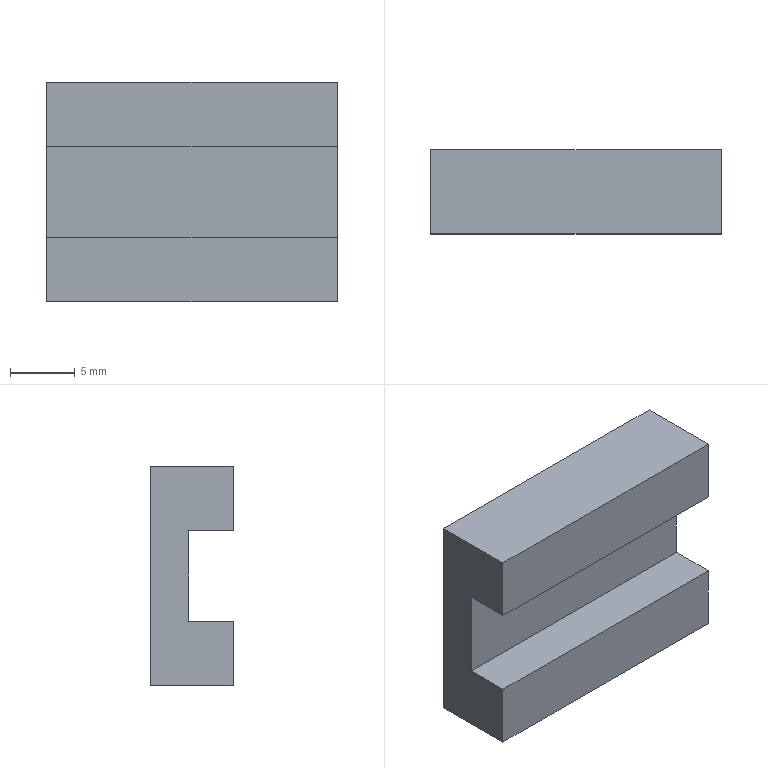Part | SolidWorks | features Extrusion 1, ICE 1 | 1 solid | 22 faces | box 22.5 x 6.5 x 17 mm | volume 1885 mm3 | plane 14 | cylinder 8 | commonest cylinder face diameters 2.635 x4 2.977 x4
STEP:
#1=CARTESIAN_POINT('',(-4.,3.047,4.441));
#2=VERTEX_POINT('',#1);
#3=CARTESIAN_POINT('',(-4.,3.047,7.076));
#4=VERTEX_POINT('',#3);
#5=CARTESIAN_POINT('',(-4.,3.047,5.759));
#6=DIRECTION('',(0.,1.,0.));
#7=DIRECTION('',(0.,0.,-1.));
#8=AXIS2_PLACEMENT_3D('',#5,#6,#7);
#9=CIRCLE('',#8,1.317);
#10=EDGE_CURVE('',#2,#4,#9,.T.);
#11=ORIENTED_EDGE('',*,*,#10,.F.);
#12=CARTESIAN_POINT('',(-4.,5.047,4.441));
#13=VERTEX_POINT('',#12);
#14=CARTESIAN_POINT('',(-4.,3.047,4.441));
#15=DIRECTION('',(0.,1.,0.));
#16=VECTOR('',#15,1000.);
#17=LINE('',#14,#16);
#18=EDGE_CURVE('',#2,#13,#17,.T.);
#19=ORIENTED_EDGE('',*,*,#18,.T.);
#20=CARTESIAN_POINT('',(-4.,5.047,7.076));
#21=VERTEX_POINT('',#20);
#22=CARTESIAN_POINT('',(-4.,5.047,5.759));
#23=DIRECTION('',(0.,1.,0.));
#24=DIRECTION('',(0.,0.,-1.));
#25=AXIS2_PLACEMENT_3D('',#22,#23,#24);
#26=CIRCLE('',#25,1.317);
#27=EDGE_CURVE('',#13,#21,#26,.T.);
#28=ORIENTED_EDGE('',*,*,#27,.T.);
#29=CARTESIAN_POINT('',(-4.,3.047,7.076));
#30=DIRECTION('',(0.,1.,0.));
#31=VECTOR('',#30,1000.);
#32=LINE('',#29,#31);
#33=EDGE_CURVE('',#4,#21,#32,.T.);
#34=ORIENTED_EDGE('',*,*,#33,.F.);
#35=EDGE_LOOP('',(#11,#19,#28,#34));
#36=FACE_OUTER_BOUND('',#35,.T.);
#37=CARTESIAN_POINT('',(-4.,3.047,5.759));
#38=DIRECTION('',(0.,1.,0.));
#39=DIRECTION('',(0.,0.,1.));
#40=AXIS2_PLACEMENT_3D('',#37,#38,#39);
#41=CYLINDRICAL_SURFACE('',#40,1.317);
#42=ADVANCED_FACE('',(#36),#41,.F.);
#43=CARTESIAN_POINT('',(4.,3.047,-7.73));
#44=VERTEX_POINT('',#43);
#45=CARTESIAN_POINT('',(4.,3.047,-4.753));
#46=VERTEX_POINT('',#45);
#47=CARTESIAN_POINT('',(4.,3.047,-6.241));
#48=DIRECTION('',(0.,1.,0.));
#49=DIRECTION('',(0.,0.,-1.));
#50=AXIS2_PLACEMENT_3D('',#47,#48,#49);
#51=CIRCLE('',#50,1.488);
#52=EDGE_CURVE('',#44,#46,#51,.T.);
#53=ORIENTED_EDGE('',*,*,#52,.F.);
#54=CARTESIAN_POINT('',(4.,5.047,-7.73));
#55=VERTEX_POINT('',#54);
#56=CARTESIAN_POINT('',(4.,3.047,-7.73));
#57=DIRECTION('',(0.,1.,0.));
#58=VECTOR('',#57,1000.);
#59=LINE('',#56,#58);
#60=EDGE_CURVE('',#44,#55,#59,.T.);
#61=ORIENTED_EDGE('',*,*,#60,.T.);
#62=CARTESIAN_POINT('',(4.,5.047,-4.753));
#63=VERTEX_POINT('',#62);
#64=CARTESIAN_POINT('',(4.,5.047,-6.241));
#65=DIRECTION('',(0.,1.,0.));
#66=DIRECTION('',(0.,0.,-1.));
#67=AXIS2_PLACEMENT_3D('',#64,#65,#66);
#68=CIRCLE('',#67,1.488);
#69=EDGE_CURVE('',#55,#63,#68,.T.);
#70=ORIENTED_EDGE('',*,*,#69,.T.);
#71=CARTESIAN_POINT('',(4.,3.047,-4.753));
#72=DIRECTION('',(0.,1.,0.));
#73=VECTOR('',#72,1000.);
#74=LINE('',#71,#73);
#75=EDGE_CURVE('',#46,#63,#74,.T.);
#76=ORIENTED_EDGE('',*,*,#75,.F.);
#77=EDGE_LOOP('',(#53,#61,#70,#76));
#78=FACE_OUTER_BOUND('',#77,.T.);
#79=CARTESIAN_POINT('',(4.,3.047,-6.241));
#80=DIRECTION('',(0.,1.,0.));
#81=DIRECTION('',(0.,0.,1.));
#82=AXIS2_PLACEMENT_3D('',#79,#80,#81);
#83=CYLINDRICAL_SURFACE('',#82,1.488);
#84=ADVANCED_FACE('',(#78),#83,.F.);
#85=CARTESIAN_POINT('',(-4.,3.047,-7.73));
#86=VERTEX_POINT('',#85);
#87=CARTESIAN_POINT('',(-4.,3.047,-4.753));
#88=VERTEX_POINT('',#87);
#89=CARTESIAN_POINT('',(-4.,3.047,-6.241));
#90=DIRECTION('',(0.,1.,0.));
#91=DIRECTION('',(0.,0.,1.));
#92=AXIS2_PLACEMENT_3D('',#89,#90,#91);
#93=CIRCLE('',#92,1.488);
#94=EDGE_CURVE('',#86,#88,#93,.T.);
#95=ORIENTED_EDGE('',*,*,#94,.F.);
#96=CARTESIAN_POINT('',(-4.,5.047,-7.73));
#97=VERTEX_POINT('',#96);
#98=CARTESIAN_POINT('',(-4.,3.047,-7.73));
#99=DIRECTION('',(0.,1.,0.));
#100=VECTOR('',#99,1000.);
#101=LINE('',#98,#100);
#102=EDGE_CURVE('',#86,#97,#101,.T.);
#103=ORIENTED_EDGE('',*,*,#102,.T.);
#104=CARTESIAN_POINT('',(-4.,5.047,-4.753));
#105=VERTEX_POINT('',#104);
#106=CARTESIAN_POINT('',(-4.,5.047,-6.241));
#107=DIRECTION('',(0.,1.,0.));
#108=DIRECTION('',(0.,0.,1.));
#109=AXIS2_PLACEMENT_3D('',#106,#107,#108);
#110=CIRCLE('',#109,1.488);
#111=EDGE_CURVE('',#97,#105,#110,.T.);
#112=ORIENTED_EDGE('',*,*,#111,.T.);
#113=CARTESIAN_POINT('',(-4.,3.047,-4.753));
#114=DIRECTION('',(0.,1.,0.));
#115=VECTOR('',#114,1000.);
#116=LINE('',#113,#115);
#117=EDGE_CURVE('',#88,#105,#116,.T.);
#118=ORIENTED_EDGE('',*,*,#117,.F.);
#119=EDGE_LOOP('',(#95,#103,#112,#118));
#120=FACE_OUTER_BOUND('',#119,.T.);
#121=CARTESIAN_POINT('',(-4.,3.047,-6.241));
#122=DIRECTION('',(0.,1.,0.));
#123=DIRECTION('',(0.,0.,1.));
#124=AXIS2_PLACEMENT_3D('',#121,#122,#123);
#125=CYLINDRICAL_SURFACE('',#124,1.488);
#126=ADVANCED_FACE('',(#120),#125,.F.);
#127=CARTESIAN_POINT('',(4.,3.047,4.441));
#128=VERTEX_POINT('',#127);
#129=CARTESIAN_POINT('',(4.,3.047,7.076));
#130=VERTEX_POINT('',#129);
#131=CARTESIAN_POINT('',(4.,3.047,5.759));
#132=DIRECTION('',(0.,1.,0.));
#133=DIRECTION('',(0.,0.,1.));
#134=AXIS2_PLACEMENT_3D('',#131,#132,#133);
#135=CIRCLE('',#134,1.317);
#136=EDGE_CURVE('',#128,#130,#135,.T.);
#137=ORIENTED_EDGE('',*,*,#136,.F.);
#138=CARTESIAN_POINT('',(4.,5.047,4.441));
#139=VERTEX_POINT('',#138);
#140=CARTESIAN_POINT('',(4.,3.047,4.441));
#141=DIRECTION('',(0.,1.,0.));
#142=VECTOR('',#141,1000.);
#143=LINE('',#140,#142);
#144=EDGE_CURVE('',#128,#139,#143,.T.);
#145=ORIENTED_EDGE('',*,*,#144,.T.);
#146=CARTESIAN_POINT('',(4.,5.047,7.076));
#147=VERTEX_POINT('',#146);
#148=CARTESIAN_POINT('',(4.,5.047,5.759));
#149=DIRECTION('',(0.,1.,0.));
#150=DIRECTION('',(0.,0.,1.));
#151=AXIS2_PLACEMENT_3D('',#148,#149,#150);
#152=CIRCLE('',#151,1.317);
#153=EDGE_CURVE('',#139,#147,#152,.T.);
#154=ORIENTED_EDGE('',*,*,#153,.T.);
#155=CARTESIAN_POINT('',(4.,3.047,7.076));
#156=DIRECTION('',(0.,1.,0.));
#157=VECTOR('',#156,1000.);
#158=LINE('',#155,#157);
#159=EDGE_CURVE('',#130,#147,#158,.T.);
#160=ORIENTED_EDGE('',*,*,#159,.F.);
#161=EDGE_LOOP('',(#137,#145,#154,#160));
#162=FACE_OUTER_BOUND('',#161,.T.);
#163=CARTESIAN_POINT('',(4.,3.047,5.759));
#164=DIRECTION('',(0.,1.,0.));
#165=DIRECTION('',(0.,0.,1.));
#166=AXIS2_PLACEMENT_3D('',#163,#164,#165);
#167=CYLINDRICAL_SURFACE('',#166,1.317);
#168=ADVANCED_FACE('',(#162),#167,.F.);
#169=CARTESIAN_POINT('',(-11.25,5.047,8.259));
#170=VERTEX_POINT('',#169);
#171=CARTESIAN_POINT('',(-11.25,-1.453,8.259));
#172=VERTEX_POINT('',#171);
#173=CARTESIAN_POINT('',(-11.25,5.047,8.259));
#174=DIRECTION('',(0.,-1.,0.));
#175=VECTOR('',#174,1000.);
#176=LINE('',#173,#175);
#177=EDGE_CURVE('',#170,#172,#176,.T.);
#178=ORIENTED_EDGE('',*,*,#177,.T.);
#179=CARTESIAN_POINT('',(11.25,-1.453,8.259));
#180=VERTEX_POINT('',#179);
#181=CARTESIAN_POINT('',(11.25,-1.453,8.259));
#182=DIRECTION('',(-1.,0.,0.));
#183=VECTOR('',#182,1000.);
#184=LINE('',#181,#183);
#185=EDGE_CURVE('',#180,#172,#184,.T.);
#186=ORIENTED_EDGE('',*,*,#185,.F.);
#187=CARTESIAN_POINT('',(11.25,5.047,8.259));
#188=VERTEX_POINT('',#187);
#189=CARTESIAN_POINT('',(11.25,5.047,8.259));
#190=DIRECTION('',(0.,-1.,0.));
#191=VECTOR('',#190,1000.);
#192=LINE('',#189,#191);
#193=EDGE_CURVE('',#188,#180,#192,.T.);
#194=ORIENTED_EDGE('',*,*,#193,.F.);
#195=CARTESIAN_POINT('',(11.25,5.047,8.259));
#196=DIRECTION('',(-1.,0.,0.));
#197=VECTOR('',#196,1000.);
#198=LINE('',#195,#197);
#199=EDGE_CURVE('',#188,#170,#198,.T.);
#200=ORIENTED_EDGE('',*,*,#199,.T.);
#201=EDGE_LOOP('',(#178,#186,#194,#200));
#202=FACE_OUTER_BOUND('',#201,.T.);
#203=CARTESIAN_POINT('',(11.25,5.047,8.259));
#204=DIRECTION('',(0.,0.,-1.));
#205=DIRECTION('',(0.,1.,0.));
#206=AXIS2_PLACEMENT_3D('',#203,#204,#205);
#207=PLANE('',#206);
#208=ADVANCED_FACE('',(#202),#207,.F.);
#209=CARTESIAN_POINT('',(-11.25,-1.453,3.259));
#210=VERTEX_POINT('',#209);
#211=CARTESIAN_POINT('',(-11.25,-1.453,8.259));
#212=DIRECTION('',(0.,0.,-1.));
#213=VECTOR('',#212,1000.);
#214=LINE('',#211,#213);
#215=EDGE_CURVE('',#172,#210,#214,.T.);
#216=ORIENTED_EDGE('',*,*,#215,.T.);
#217=CARTESIAN_POINT('',(11.25,-1.453,3.259));
#218=VERTEX_POINT('',#217);
#219=CARTESIAN_POINT('',(11.25,-1.453,3.259));
#220=DIRECTION('',(-1.,0.,0.));
#221=VECTOR('',#220,1000.);
#222=LINE('',#219,#221);
#223=EDGE_CURVE('',#218,#210,#222,.T.);
#224=ORIENTED_EDGE('',*,*,#223,.F.);
#225=CARTESIAN_POINT('',(11.25,-1.453,8.259));
#226=DIRECTION('',(0.,0.,-1.));
#227=VECTOR('',#226,1000.);
#228=LINE('',#225,#227);
#229=EDGE_CURVE('',#180,#218,#228,.T.);
#230=ORIENTED_EDGE('',*,*,#229,.F.);
#231=ORIENTED_EDGE('',*,*,#185,.T.);
#232=EDGE_LOOP('',(#216,#224,#230,#231));
#233=FACE_OUTER_BOUND('',#232,.T.);
#234=CARTESIAN_POINT('',(11.25,-1.453,8.259));
#235=DIRECTION('',(0.,1.,0.));
#236=DIRECTION('',(0.,0.,1.));
#237=AXIS2_PLACEMENT_3D('',#234,#235,#236);
#238=PLANE('',#237);
#239=ADVANCED_FACE('',(#233),#238,.F.);
#240=CARTESIAN_POINT('',(-11.25,2.047,3.259));
#241=VERTEX_POINT('',#240);
#242=CARTESIAN_POINT('',(-11.25,-1.453,3.259));
#243=DIRECTION('',(0.,1.,0.));
#244=VECTOR('',#243,1000.);
#245=LINE('',#242,#244);
#246=EDGE_CURVE('',#210,#241,#245,.T.);
#247=ORIENTED_EDGE('',*,*,#246,.T.);
#248=CARTESIAN_POINT('',(11.25,2.047,3.259));
#249=VERTEX_POINT('',#248);
#250=CARTESIAN_POINT('',(11.25,2.047,3.259));
#251=DIRECTION('',(-1.,0.,0.));
#252=VECTOR('',#251,1000.);
#253=LINE('',#250,#252);
#254=EDGE_CURVE('',#249,#241,#253,.T.);
#255=ORIENTED_EDGE('',*,*,#254,.F.);
#256=CARTESIAN_POINT('',(11.25,-1.453,3.259));
#257=DIRECTION('',(0.,1.,0.));
#258=VECTOR('',#257,1000.);
#259=LINE('',#256,#258);
#260=EDGE_CURVE('',#218,#249,#259,.T.);
#261=ORIENTED_EDGE('',*,*,#260,.F.);
#262=ORIENTED_EDGE('',*,*,#223,.T.);
#263=EDGE_LOOP('',(#247,#255,#261,#262));
#264=FACE_OUTER_BOUND('',#263,.T.);
#265=CARTESIAN_POINT('',(11.25,-1.453,3.259));
#266=DIRECTION('',(0.,0.,1.));
#267=DIRECTION('',(1.,0.,0.));
#268=AXIS2_PLACEMENT_3D('',#265,#266,#267);
#269=PLANE('',#268);
#270=ADVANCED_FACE('',(#264),#269,.F.);
#271=CARTESIAN_POINT('',(-11.25,2.047,-3.741));
#272=VERTEX_POINT('',#271);
#273=CARTESIAN_POINT('',(-11.25,2.047,3.259));
#274=DIRECTION('',(0.,0.,-1.));
#275=VECTOR('',#274,1000.);
#276=LINE('',#273,#275);
#277=EDGE_CURVE('',#241,#272,#276,.T.);
#278=ORIENTED_EDGE('',*,*,#277,.T.);
#279=CARTESIAN_POINT('',(11.25,2.047,-3.741));
#280=VERTEX_POINT('',#279);
#281=CARTESIAN_POINT('',(11.25,2.047,-3.741));
#282=DIRECTION('',(-1.,0.,0.));
#283=VECTOR('',#282,1000.);
#284=LINE('',#281,#283);
#285=EDGE_CURVE('',#280,#272,#284,.T.);
#286=ORIENTED_EDGE('',*,*,#285,.F.);
#287=CARTESIAN_POINT('',(11.25,2.047,3.259));
#288=DIRECTION('',(0.,0.,-1.));
#289=VECTOR('',#288,1000.);
#290=LINE('',#287,#289);
#291=EDGE_CURVE('',#249,#280,#290,.T.);
#292=ORIENTED_EDGE('',*,*,#291,.F.);
#293=ORIENTED_EDGE('',*,*,#254,.T.);
#294=EDGE_LOOP('',(#278,#286,#292,#293));
#295=FACE_OUTER_BOUND('',#294,.T.);
#296=CARTESIAN_POINT('',(11.25,2.047,3.259));
#297=DIRECTION('',(0.,1.,0.));
#298=DIRECTION('',(0.,0.,1.));
#299=AXIS2_PLACEMENT_3D('',#296,#297,#298);
#300=PLANE('',#299);
#301=ADVANCED_FACE('',(#295),#300,.F.);
#302=CARTESIAN_POINT('',(-11.25,-1.453,-3.741));
#303=VERTEX_POINT('',#302);
#304=CARTESIAN_POINT('',(-11.25,2.047,-3.741));
#305=DIRECTION('',(0.,-1.,0.));
#306=VECTOR('',#305,1000.);
#307=LINE('',#304,#306);
#308=EDGE_CURVE('',#272,#303,#307,.T.);
#309=ORIENTED_EDGE('',*,*,#308,.T.);
#310=CARTESIAN_POINT('',(11.25,-1.453,-3.741));
#311=VERTEX_POINT('',#310);
#312=CARTESIAN_POINT('',(11.25,-1.453,-3.741));
#313=DIRECTION('',(-1.,0.,0.));
#314=VECTOR('',#313,1000.);
#315=LINE('',#312,#314);
#316=EDGE_CURVE('',#311,#303,#315,.T.);
#317=ORIENTED_EDGE('',*,*,#316,.F.);
#318=CARTESIAN_POINT('',(11.25,2.047,-3.741));
#319=DIRECTION('',(0.,-1.,0.));
#320=VECTOR('',#319,1000.);
#321=LINE('',#318,#320);
#322=EDGE_CURVE('',#280,#311,#321,.T.);
#323=ORIENTED_EDGE('',*,*,#322,.F.);
#324=ORIENTED_EDGE('',*,*,#285,.T.);
#325=EDGE_LOOP('',(#309,#317,#323,#324));
#326=FACE_OUTER_BOUND('',#325,.T.);
#327=CARTESIAN_POINT('',(11.25,2.047,-3.741));
#328=DIRECTION('',(0.,0.,-1.));
#329=DIRECTION('',(0.,1.,0.));
#330=AXIS2_PLACEMENT_3D('',#327,#328,#329);
#331=PLANE('',#330);
#332=ADVANCED_FACE('',(#326),#331,.F.);
#333=CARTESIAN_POINT('',(-11.25,-1.453,-8.741));
#334=VERTEX_POINT('',#333);
#335=CARTESIAN_POINT('',(-11.25,-1.453,-3.741));
#336=DIRECTION('',(0.,0.,-1.));
#337=VECTOR('',#336,1000.);
#338=LINE('',#335,#337);
#339=EDGE_CURVE('',#303,#334,#338,.T.);
#340=ORIENTED_EDGE('',*,*,#339,.T.);
#341=CARTESIAN_POINT('',(11.25,-1.453,-8.741));
#342=VERTEX_POINT('',#341);
#343=CARTESIAN_POINT('',(11.25,-1.453,-8.741));
#344=DIRECTION('',(-1.,0.,0.));
#345=VECTOR('',#344,1000.);
#346=LINE('',#343,#345);
#347=EDGE_CURVE('',#342,#334,#346,.T.);
#348=ORIENTED_EDGE('',*,*,#347,.F.);
#349=CARTESIAN_POINT('',(11.25,-1.453,-3.741));
#350=DIRECTION('',(0.,0.,-1.));
#351=VECTOR('',#350,1000.);
#352=LINE('',#349,#351);
#353=EDGE_CURVE('',#311,#342,#352,.T.);
#354=ORIENTED_EDGE('',*,*,#353,.F.);
#355=ORIENTED_EDGE('',*,*,#316,.T.);
#356=EDGE_LOOP('',(#340,#348,#354,#355));
#357=FACE_OUTER_BOUND('',#356,.T.);
#358=CARTESIAN_POINT('',(11.25,-1.453,-3.741));
#359=DIRECTION('',(0.,1.,0.));
#360=DIRECTION('',(0.,0.,1.));
#361=AXIS2_PLACEMENT_3D('',#358,#359,#360);
#362=PLANE('',#361);
#363=ADVANCED_FACE('',(#357),#362,.F.);
#364=CARTESIAN_POINT('',(-11.25,5.047,-8.741));
#365=VERTEX_POINT('',#364);
#366=CARTESIAN_POINT('',(-11.25,5.047,-8.741));
#367=DIRECTION('',(0.,1.,0.));
#368=VECTOR('',#367,1000.);
#369=LINE('',#366,#368);
#370=EDGE_CURVE('',#334,#365,#369,.T.);
#371=ORIENTED_EDGE('',*,*,#370,.T.);
#372=CARTESIAN_POINT('',(11.25,5.047,-8.741));
#373=VERTEX_POINT('',#372);
#374=CARTESIAN_POINT('',(11.25,5.047,-8.741));
#375=DIRECTION('',(-1.,0.,0.));
#376=VECTOR('',#375,1000.);
#377=LINE('',#374,#376);
#378=EDGE_CURVE('',#373,#365,#377,.T.);
#379=ORIENTED_EDGE('',*,*,#378,.F.);
#380=CARTESIAN_POINT('',(11.25,5.047,-8.741));
#381=DIRECTION('',(0.,1.,0.));
#382=VECTOR('',#381,1000.);
#383=LINE('',#380,#382);
#384=EDGE_CURVE('',#342,#373,#383,.T.);
#385=ORIENTED_EDGE('',*,*,#384,.F.);
#386=ORIENTED_EDGE('',*,*,#347,.T.);
#387=EDGE_LOOP('',(#371,#379,#385,#386));
#388=FACE_OUTER_BOUND('',#387,.T.);
#389=CARTESIAN_POINT('',(11.25,5.047,-8.741));
#390=DIRECTION('',(0.,0.,1.));
#391=DIRECTION('',(1.,0.,0.));
#392=AXIS2_PLACEMENT_3D('',#389,#390,#391);
#393=PLANE('',#392);
#394=ADVANCED_FACE('',(#388),#393,.F.);
#395=CARTESIAN_POINT('',(-4.,5.047,5.759));
#396=DIRECTION('',(0.,1.,0.));
#397=DIRECTION('',(0.,0.,-1.));
#398=AXIS2_PLACEMENT_3D('',#395,#396,#397);
#399=CIRCLE('',#398,1.317);
#400=EDGE_CURVE('',#21,#13,#399,.T.);
#401=ORIENTED_EDGE('',*,*,#400,.F.);
#402=ORIENTED_EDGE('',*,*,#27,.F.);
#403=EDGE_LOOP('',(#401,#402));
#404=FACE_BOUND('',#403,.T.);
#405=CARTESIAN_POINT('',(4.,5.047,-6.241));
#406=DIRECTION('',(0.,1.,0.));
#407=DIRECTION('',(0.,0.,-1.));
#408=AXIS2_PLACEMENT_3D('',#405,#406,#407);
#409=CIRCLE('',#408,1.488);
#410=EDGE_CURVE('',#63,#55,#409,.T.);
#411=ORIENTED_EDGE('',*,*,#410,.F.);
#412=ORIENTED_EDGE('',*,*,#69,.F.);
#413=EDGE_LOOP('',(#411,#412));
#414=FACE_BOUND('',#413,.T.);
#415=CARTESIAN_POINT('',(-4.,5.047,-6.241));
#416=DIRECTION('',(0.,1.,0.));
#417=DIRECTION('',(0.,0.,1.));
#418=AXIS2_PLACEMENT_3D('',#415,#416,#417);
#419=CIRCLE('',#418,1.488);
#420=EDGE_CURVE('',#105,#97,#419,.T.);
#421=ORIENTED_EDGE('',*,*,#420,.F.);
#422=ORIENTED_EDGE('',*,*,#111,.F.);
#423=EDGE_LOOP('',(#421,#422));
#424=FACE_BOUND('',#423,.T.);
#425=CARTESIAN_POINT('',(4.,5.047,5.759));
#426=DIRECTION('',(0.,1.,0.));
#427=DIRECTION('',(0.,0.,1.));
#428=AXIS2_PLACEMENT_3D('',#425,#426,#427);
#429=CIRCLE('',#428,1.317);
#430=EDGE_CURVE('',#147,#139,#429,.T.);
#431=ORIENTED_EDGE('',*,*,#430,.F.);
#432=ORIENTED_EDGE('',*,*,#153,.F.);
#433=EDGE_LOOP('',(#431,#432));
#434=FACE_BOUND('',#433,.T.);
#435=CARTESIAN_POINT('',(-11.25,5.047,8.259));
#436=DIRECTION('',(0.,0.,1.));
#437=VECTOR('',#436,1000.);
#438=LINE('',#435,#437);
#439=EDGE_CURVE('',#365,#170,#438,.T.);
#440=ORIENTED_EDGE('',*,*,#439,.T.);
#441=ORIENTED_EDGE('',*,*,#199,.F.);
#442=CARTESIAN_POINT('',(11.25,5.047,8.259));
#443=DIRECTION('',(0.,0.,1.));
#444=VECTOR('',#443,1000.);
#445=LINE('',#442,#444);
#446=EDGE_CURVE('',#373,#188,#445,.T.);
#447=ORIENTED_EDGE('',*,*,#446,.F.);
#448=ORIENTED_EDGE('',*,*,#378,.T.);
#449=EDGE_LOOP('',(#440,#441,#447,#448));
#450=FACE_OUTER_BOUND('',#449,.T.);
#451=CARTESIAN_POINT('',(11.25,5.047,8.259));
#452=DIRECTION('',(0.,-1.,0.));
#453=DIRECTION('',(0.,0.,-1.));
#454=AXIS2_PLACEMENT_3D('',#451,#452,#453);
#455=PLANE('',#454);
#456=ADVANCED_FACE('',(#404,#414,#424,#434,#450),#455,.F.);
#457=ORIENTED_EDGE('',*,*,#193,.T.);
#458=ORIENTED_EDGE('',*,*,#229,.T.);
#459=ORIENTED_EDGE('',*,*,#260,.T.);
#460=ORIENTED_EDGE('',*,*,#291,.T.);
#461=ORIENTED_EDGE('',*,*,#322,.T.);
#462=ORIENTED_EDGE('',*,*,#353,.T.);
#463=ORIENTED_EDGE('',*,*,#384,.T.);
#464=ORIENTED_EDGE('',*,*,#446,.T.);
#465=EDGE_LOOP('',(#457,#458,#459,#460,#461,#462,#463,#464));
#466=FACE_OUTER_BOUND('',#465,.T.);
#467=CARTESIAN_POINT('',(11.25,0.,0.));
#468=DIRECTION('',(1.,0.,0.));
#469=DIRECTION('',(0.,0.,-1.));
#470=AXIS2_PLACEMENT_3D('',#467,#468,#469);
#471=PLANE('',#470);
#472=ADVANCED_FACE('',(#466),#471,.T.);
#473=ORIENTED_EDGE('',*,*,#177,.F.);
#474=ORIENTED_EDGE('',*,*,#439,.F.);
#475=ORIENTED_EDGE('',*,*,#370,.F.);
#476=ORIENTED_EDGE('',*,*,#339,.F.);
#477=ORIENTED_EDGE('',*,*,#308,.F.);
#478=ORIENTED_EDGE('',*,*,#277,.F.);
#479=ORIENTED_EDGE('',*,*,#246,.F.);
#480=ORIENTED_EDGE('',*,*,#215,.F.);
#481=EDGE_LOOP('',(#473,#474,#475,#476,#477,#478,#479,#480));
#482=FACE_OUTER_BOUND('',#481,.T.);
#483=CARTESIAN_POINT('',(-11.25,0.,0.));
#484=DIRECTION('',(1.,0.,0.));
#485=DIRECTION('',(0.,0.,-1.));
#486=AXIS2_PLACEMENT_3D('',#483,#484,#485);
#487=PLANE('',#486);
#488=ADVANCED_FACE('',(#482),#487,.F.);
#489=ORIENTED_EDGE('',*,*,#144,.F.);
#490=CARTESIAN_POINT('',(4.,3.047,5.759));
#491=DIRECTION('',(0.,1.,0.));
#492=DIRECTION('',(0.,0.,1.));
#493=AXIS2_PLACEMENT_3D('',#490,#491,#492);
#494=CIRCLE('',#493,1.317);
#495=EDGE_CURVE('',#130,#128,#494,.T.);
#496=ORIENTED_EDGE('',*,*,#495,.F.);
#497=ORIENTED_EDGE('',*,*,#159,.T.);
#498=ORIENTED_EDGE('',*,*,#430,.T.);
#499=EDGE_LOOP('',(#489,#496,#497,#498));
#500=FACE_OUTER_BOUND('',#499,.T.);
#501=CARTESIAN_POINT('',(4.,3.047,5.759));
#502=DIRECTION('',(0.,1.,0.));
#503=DIRECTION('',(0.,0.,1.));
#504=AXIS2_PLACEMENT_3D('',#501,#502,#503);
#505=CYLINDRICAL_SURFACE('',#504,1.317);
#506=ADVANCED_FACE('',(#500),#505,.F.);
#507=ORIENTED_EDGE('',*,*,#495,.T.);
#508=ORIENTED_EDGE('',*,*,#136,.T.);
#509=EDGE_LOOP('',(#507,#508));
#510=FACE_OUTER_BOUND('',#509,.T.);
#511=CARTESIAN_POINT('',(4.,3.047,5.759));
#512=DIRECTION('',(0.,1.,0.));
#513=DIRECTION('',(0.,0.,1.));
#514=AXIS2_PLACEMENT_3D('',#511,#512,#513);
#515=PLANE('',#514);
#516=ADVANCED_FACE('',(#510),#515,.T.);
#517=ORIENTED_EDGE('',*,*,#102,.F.);
#518=CARTESIAN_POINT('',(-4.,3.047,-6.241));
#519=DIRECTION('',(0.,1.,0.));
#520=DIRECTION('',(0.,0.,1.));
#521=AXIS2_PLACEMENT_3D('',#518,#519,#520);
#522=CIRCLE('',#521,1.488);
#523=EDGE_CURVE('',#88,#86,#522,.T.);
#524=ORIENTED_EDGE('',*,*,#523,.F.);
#525=ORIENTED_EDGE('',*,*,#117,.T.);
#526=ORIENTED_EDGE('',*,*,#420,.T.);
#527=EDGE_LOOP('',(#517,#524,#525,#526));
#528=FACE_OUTER_BOUND('',#527,.T.);
#529=CARTESIAN_POINT('',(-4.,3.047,-6.241));
#530=DIRECTION('',(0.,1.,0.));
#531=DIRECTION('',(0.,0.,1.));
#532=AXIS2_PLACEMENT_3D('',#529,#530,#531);
#533=CYLINDRICAL_SURFACE('',#532,1.488);
#534=ADVANCED_FACE('',(#528),#533,.F.);
#535=ORIENTED_EDGE('',*,*,#523,.T.);
#536=ORIENTED_EDGE('',*,*,#94,.T.);
#537=EDGE_LOOP('',(#535,#536));
#538=FACE_OUTER_BOUND('',#537,.T.);
#539=CARTESIAN_POINT('',(-4.,3.047,-6.241));
#540=DIRECTION('',(0.,1.,0.));
#541=DIRECTION('',(0.,0.,1.));
#542=AXIS2_PLACEMENT_3D('',#539,#540,#541);
#543=PLANE('',#542);
#544=ADVANCED_FACE('',(#538),#543,.T.);
#545=ORIENTED_EDGE('',*,*,#60,.F.);
#546=CARTESIAN_POINT('',(4.,3.047,-6.241));
#547=DIRECTION('',(0.,1.,0.));
#548=DIRECTION('',(0.,0.,-1.));
#549=AXIS2_PLACEMENT_3D('',#546,#547,#548);
#550=CIRCLE('',#549,1.488);
#551=EDGE_CURVE('',#46,#44,#550,.T.);
#552=ORIENTED_EDGE('',*,*,#551,.F.);
#553=ORIENTED_EDGE('',*,*,#75,.T.);
#554=ORIENTED_EDGE('',*,*,#410,.T.);
#555=EDGE_LOOP('',(#545,#552,#553,#554));
#556=FACE_OUTER_BOUND('',#555,.T.);
#557=CARTESIAN_POINT('',(4.,3.047,-6.241));
#558=DIRECTION('',(0.,1.,0.));
#559=DIRECTION('',(0.,0.,1.));
#560=AXIS2_PLACEMENT_3D('',#557,#558,#559);
#561=CYLINDRICAL_SURFACE('',#560,1.488);
#562=ADVANCED_FACE('',(#556),#561,.F.);
#563=ORIENTED_EDGE('',*,*,#551,.T.);
#564=ORIENTED_EDGE('',*,*,#52,.T.);
#565=EDGE_LOOP('',(#563,#564));
#566=FACE_OUTER_BOUND('',#565,.T.);
#567=CARTESIAN_POINT('',(4.,3.047,-6.241));
#568=DIRECTION('',(0.,-1.,0.));
#569=DIRECTION('',(0.,0.,-1.));
#570=AXIS2_PLACEMENT_3D('',#567,#568,#569);
#571=PLANE('',#570);
#572=ADVANCED_FACE('',(#566),#571,.F.);
#573=ORIENTED_EDGE('',*,*,#18,.F.);
#574=CARTESIAN_POINT('',(-4.,3.047,5.759));
#575=DIRECTION('',(0.,1.,0.));
#576=DIRECTION('',(0.,0.,-1.));
#577=AXIS2_PLACEMENT_3D('',#574,#575,#576);
#578=CIRCLE('',#577,1.317);
#579=EDGE_CURVE('',#4,#2,#578,.T.);
#580=ORIENTED_EDGE('',*,*,#579,.F.);
#581=ORIENTED_EDGE('',*,*,#33,.T.);
#582=ORIENTED_EDGE('',*,*,#400,.T.);
#583=EDGE_LOOP('',(#573,#580,#581,#582));
#584=FACE_OUTER_BOUND('',#583,.T.);
#585=CARTESIAN_POINT('',(-4.,3.047,5.759));
#586=DIRECTION('',(0.,1.,0.));
#587=DIRECTION('',(0.,0.,1.));
#588=AXIS2_PLACEMENT_3D('',#585,#586,#587);
#589=CYLINDRICAL_SURFACE('',#588,1.317);
#590=ADVANCED_FACE('',(#584),#589,.F.);
#591=ORIENTED_EDGE('',*,*,#579,.T.);
#592=ORIENTED_EDGE('',*,*,#10,.T.);
#593=EDGE_LOOP('',(#591,#592));
#594=FACE_OUTER_BOUND('',#593,.T.);
#595=CARTESIAN_POINT('',(-4.,3.047,5.759));
#596=DIRECTION('',(0.,-1.,0.));
#597=DIRECTION('',(0.,0.,-1.));
#598=AXIS2_PLACEMENT_3D('',#595,#596,#597);
#599=PLANE('',#598);
#600=ADVANCED_FACE('',(#594),#599,.F.);
#601=CLOSED_SHELL('',(#42,#84,#126,#168,#208,#239,#270,#301,#332,#363,#394,#456,#472,#488,#506,#516,#534,#544,#562,#572,#590,#600));
#602=MANIFOLD_SOLID_BREP('',#601);
#603=CARTESIAN_POINT('',(0.,0.,0.));
#604=DIRECTION('',(0.,0.,1.));
#605=DIRECTION('',(1.,0.,0.));
#606=AXIS2_PLACEMENT_3D('',#603,#604,#605);
#607=(LENGTH_UNIT()NAMED_UNIT(*)SI_UNIT(.MILLI.,.METRE.));
#608=UNCERTAINTY_MEASURE_WITH_UNIT(LENGTH_MEASURE(0.00001),#607,'','');
#609=(NAMED_UNIT(*)PLANE_ANGLE_UNIT()SI_UNIT($,.RADIAN.));
#610=(NAMED_UNIT(*)SI_UNIT($,.STERADIAN.)SOLID_ANGLE_UNIT());
#611=(GEOMETRIC_REPRESENTATION_CONTEXT(3)GLOBAL_UNCERTAINTY_ASSIGNED_CONTEXT((#608))GLOBAL_UNIT_ASSIGNED_CONTEXT((#607,#609,#610))REPRESENTATION_CONTEXT('',''));
#612=ADVANCED_BREP_SHAPE_REPRESENTATION('',(#602,#606),#611);